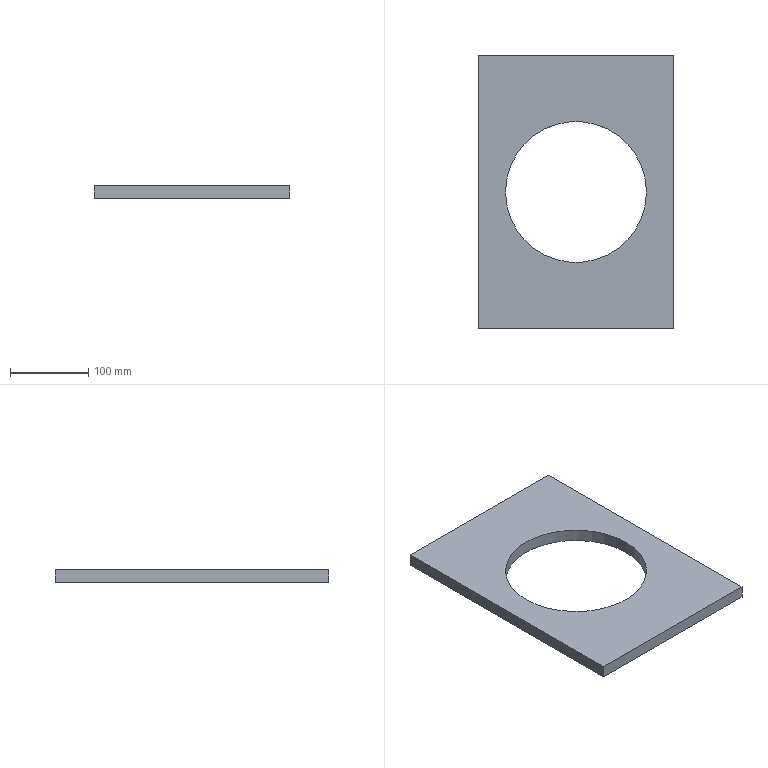Part | SolidWorks | features Extrusion 1 | 1 solid | 8 faces | box 250 x 350 x 16 mm | volume 992850 mm3 | plane 6 | cylinder 2 | commonest cylinder face diameters 180 x2
STEP:
#1=CARTESIAN_POINT('',(-90.,0.,16.));
#2=VERTEX_POINT('',#1);
#3=CARTESIAN_POINT('',(90.,0.,16.));
#4=VERTEX_POINT('',#3);
#5=CARTESIAN_POINT('',(0.,0.,16.));
#6=DIRECTION('',(0.,0.,1.));
#7=DIRECTION('',(1.,0.,0.));
#8=AXIS2_PLACEMENT_3D('',#5,#6,#7);
#9=CIRCLE('',#8,90.);
#10=EDGE_CURVE('',#2,#4,#9,.T.);
#11=ORIENTED_EDGE('',*,*,#10,.T.);
#12=CARTESIAN_POINT('',(90.,0.,0.));
#13=VERTEX_POINT('',#12);
#14=CARTESIAN_POINT('',(90.,0.,16.));
#15=DIRECTION('',(0.,0.,-1.));
#16=VECTOR('',#15,1000.);
#17=LINE('',#14,#16);
#18=EDGE_CURVE('',#4,#13,#17,.T.);
#19=ORIENTED_EDGE('',*,*,#18,.T.);
#20=CARTESIAN_POINT('',(-90.,0.,0.));
#21=VERTEX_POINT('',#20);
#22=CARTESIAN_POINT('',(0.,0.,0.));
#23=DIRECTION('',(0.,0.,1.));
#24=DIRECTION('',(1.,0.,0.));
#25=AXIS2_PLACEMENT_3D('',#22,#23,#24);
#26=CIRCLE('',#25,90.);
#27=EDGE_CURVE('',#21,#13,#26,.T.);
#28=ORIENTED_EDGE('',*,*,#27,.F.);
#29=CARTESIAN_POINT('',(-90.,0.,16.));
#30=DIRECTION('',(0.,0.,-1.));
#31=VECTOR('',#30,1000.);
#32=LINE('',#29,#31);
#33=EDGE_CURVE('',#2,#21,#32,.T.);
#34=ORIENTED_EDGE('',*,*,#33,.F.);
#35=EDGE_LOOP('',(#11,#19,#28,#34));
#36=FACE_OUTER_BOUND('',#35,.T.);
#37=CARTESIAN_POINT('',(0.,0.,16.));
#38=DIRECTION('',(0.,0.,-1.));
#39=DIRECTION('',(-1.,0.,0.));
#40=AXIS2_PLACEMENT_3D('',#37,#38,#39);
#41=CYLINDRICAL_SURFACE('',#40,90.);
#42=ADVANCED_FACE('',(#36),#41,.F.);
#43=CARTESIAN_POINT('',(-125.,175.,16.));
#44=VERTEX_POINT('',#43);
#45=CARTESIAN_POINT('',(-125.,-175.,16.));
#46=VERTEX_POINT('',#45);
#47=CARTESIAN_POINT('',(-125.,-175.,16.));
#48=DIRECTION('',(0.,-1.,0.));
#49=VECTOR('',#48,1000.);
#50=LINE('',#47,#49);
#51=EDGE_CURVE('',#44,#46,#50,.T.);
#52=ORIENTED_EDGE('',*,*,#51,.T.);
#53=CARTESIAN_POINT('',(125.,-175.,16.));
#54=VERTEX_POINT('',#53);
#55=CARTESIAN_POINT('',(125.,-175.,16.));
#56=DIRECTION('',(1.,0.,0.));
#57=VECTOR('',#56,1000.);
#58=LINE('',#55,#57);
#59=EDGE_CURVE('',#46,#54,#58,.T.);
#60=ORIENTED_EDGE('',*,*,#59,.T.);
#61=CARTESIAN_POINT('',(125.,175.,16.));
#62=VERTEX_POINT('',#61);
#63=CARTESIAN_POINT('',(125.,-175.,16.));
#64=DIRECTION('',(0.,1.,0.));
#65=VECTOR('',#64,1000.);
#66=LINE('',#63,#65);
#67=EDGE_CURVE('',#54,#62,#66,.T.);
#68=ORIENTED_EDGE('',*,*,#67,.T.);
#69=CARTESIAN_POINT('',(125.,175.,16.));
#70=DIRECTION('',(-1.,0.,0.));
#71=VECTOR('',#70,1000.);
#72=LINE('',#69,#71);
#73=EDGE_CURVE('',#62,#44,#72,.T.);
#74=ORIENTED_EDGE('',*,*,#73,.T.);
#75=EDGE_LOOP('',(#52,#60,#68,#74));
#76=FACE_OUTER_BOUND('',#75,.T.);
#77=ORIENTED_EDGE('',*,*,#10,.F.);
#78=CARTESIAN_POINT('',(0.,0.,16.));
#79=DIRECTION('',(0.,0.,1.));
#80=DIRECTION('',(1.,0.,0.));
#81=AXIS2_PLACEMENT_3D('',#78,#79,#80);
#82=CIRCLE('',#81,90.);
#83=EDGE_CURVE('',#4,#2,#82,.T.);
#84=ORIENTED_EDGE('',*,*,#83,.F.);
#85=EDGE_LOOP('',(#77,#84));
#86=FACE_BOUND('',#85,.T.);
#87=CARTESIAN_POINT('',(0.,0.,16.));
#88=DIRECTION('',(0.,0.,1.));
#89=DIRECTION('',(1.,0.,0.));
#90=AXIS2_PLACEMENT_3D('',#87,#88,#89);
#91=PLANE('',#90);
#92=ADVANCED_FACE('',(#76,#86),#91,.T.);
#93=CARTESIAN_POINT('',(-125.,175.,0.));
#94=VERTEX_POINT('',#93);
#95=CARTESIAN_POINT('',(-125.,-175.,0.));
#96=VERTEX_POINT('',#95);
#97=CARTESIAN_POINT('',(-125.,-175.,0.));
#98=DIRECTION('',(0.,-1.,0.));
#99=VECTOR('',#98,1000.);
#100=LINE('',#97,#99);
#101=EDGE_CURVE('',#94,#96,#100,.T.);
#102=ORIENTED_EDGE('',*,*,#101,.F.);
#103=CARTESIAN_POINT('',(125.,175.,0.));
#104=VERTEX_POINT('',#103);
#105=CARTESIAN_POINT('',(125.,175.,0.));
#106=DIRECTION('',(-1.,0.,0.));
#107=VECTOR('',#106,1000.);
#108=LINE('',#105,#107);
#109=EDGE_CURVE('',#104,#94,#108,.T.);
#110=ORIENTED_EDGE('',*,*,#109,.F.);
#111=CARTESIAN_POINT('',(125.,-175.,0.));
#112=VERTEX_POINT('',#111);
#113=CARTESIAN_POINT('',(125.,-175.,0.));
#114=DIRECTION('',(0.,1.,0.));
#115=VECTOR('',#114,1000.);
#116=LINE('',#113,#115);
#117=EDGE_CURVE('',#112,#104,#116,.T.);
#118=ORIENTED_EDGE('',*,*,#117,.F.);
#119=CARTESIAN_POINT('',(125.,-175.,0.));
#120=DIRECTION('',(1.,0.,0.));
#121=VECTOR('',#120,1000.);
#122=LINE('',#119,#121);
#123=EDGE_CURVE('',#96,#112,#122,.T.);
#124=ORIENTED_EDGE('',*,*,#123,.F.);
#125=EDGE_LOOP('',(#102,#110,#118,#124));
#126=FACE_OUTER_BOUND('',#125,.T.);
#127=ORIENTED_EDGE('',*,*,#27,.T.);
#128=CARTESIAN_POINT('',(0.,0.,0.));
#129=DIRECTION('',(0.,0.,1.));
#130=DIRECTION('',(1.,0.,0.));
#131=AXIS2_PLACEMENT_3D('',#128,#129,#130);
#132=CIRCLE('',#131,90.);
#133=EDGE_CURVE('',#13,#21,#132,.T.);
#134=ORIENTED_EDGE('',*,*,#133,.T.);
#135=EDGE_LOOP('',(#127,#134));
#136=FACE_BOUND('',#135,.T.);
#137=CARTESIAN_POINT('',(0.,0.,0.));
#138=DIRECTION('',(0.,0.,1.));
#139=DIRECTION('',(1.,0.,0.));
#140=AXIS2_PLACEMENT_3D('',#137,#138,#139);
#141=PLANE('',#140);
#142=ADVANCED_FACE('',(#126,#136),#141,.F.);
#143=ORIENTED_EDGE('',*,*,#101,.T.);
#144=CARTESIAN_POINT('',(-125.,-175.,16.));
#145=DIRECTION('',(0.,0.,-1.));
#146=VECTOR('',#145,1000.);
#147=LINE('',#144,#146);
#148=EDGE_CURVE('',#46,#96,#147,.T.);
#149=ORIENTED_EDGE('',*,*,#148,.F.);
#150=ORIENTED_EDGE('',*,*,#51,.F.);
#151=CARTESIAN_POINT('',(-125.,175.,16.));
#152=DIRECTION('',(0.,0.,-1.));
#153=VECTOR('',#152,1000.);
#154=LINE('',#151,#153);
#155=EDGE_CURVE('',#44,#94,#154,.T.);
#156=ORIENTED_EDGE('',*,*,#155,.T.);
#157=EDGE_LOOP('',(#143,#149,#150,#156));
#158=FACE_OUTER_BOUND('',#157,.T.);
#159=CARTESIAN_POINT('',(-125.,-175.,16.));
#160=DIRECTION('',(1.,0.,0.));
#161=DIRECTION('',(0.,0.,-1.));
#162=AXIS2_PLACEMENT_3D('',#159,#160,#161);
#163=PLANE('',#162);
#164=ADVANCED_FACE('',(#158),#163,.F.);
#165=ORIENTED_EDGE('',*,*,#123,.T.);
#166=CARTESIAN_POINT('',(125.,-175.,16.));
#167=DIRECTION('',(0.,0.,-1.));
#168=VECTOR('',#167,1000.);
#169=LINE('',#166,#168);
#170=EDGE_CURVE('',#54,#112,#169,.T.);
#171=ORIENTED_EDGE('',*,*,#170,.F.);
#172=ORIENTED_EDGE('',*,*,#59,.F.);
#173=ORIENTED_EDGE('',*,*,#148,.T.);
#174=EDGE_LOOP('',(#165,#171,#172,#173));
#175=FACE_OUTER_BOUND('',#174,.T.);
#176=CARTESIAN_POINT('',(125.,-175.,16.));
#177=DIRECTION('',(0.,1.,0.));
#178=DIRECTION('',(-1.,0.,0.));
#179=AXIS2_PLACEMENT_3D('',#176,#177,#178);
#180=PLANE('',#179);
#181=ADVANCED_FACE('',(#175),#180,.F.);
#182=ORIENTED_EDGE('',*,*,#117,.T.);
#183=CARTESIAN_POINT('',(125.,175.,16.));
#184=DIRECTION('',(0.,0.,-1.));
#185=VECTOR('',#184,1000.);
#186=LINE('',#183,#185);
#187=EDGE_CURVE('',#62,#104,#186,.T.);
#188=ORIENTED_EDGE('',*,*,#187,.F.);
#189=ORIENTED_EDGE('',*,*,#67,.F.);
#190=ORIENTED_EDGE('',*,*,#170,.T.);
#191=EDGE_LOOP('',(#182,#188,#189,#190));
#192=FACE_OUTER_BOUND('',#191,.T.);
#193=CARTESIAN_POINT('',(125.,-175.,16.));
#194=DIRECTION('',(-1.,0.,0.));
#195=DIRECTION('',(0.,0.,1.));
#196=AXIS2_PLACEMENT_3D('',#193,#194,#195);
#197=PLANE('',#196);
#198=ADVANCED_FACE('',(#192),#197,.F.);
#199=ORIENTED_EDGE('',*,*,#109,.T.);
#200=ORIENTED_EDGE('',*,*,#155,.F.);
#201=ORIENTED_EDGE('',*,*,#73,.F.);
#202=ORIENTED_EDGE('',*,*,#187,.T.);
#203=EDGE_LOOP('',(#199,#200,#201,#202));
#204=FACE_OUTER_BOUND('',#203,.T.);
#205=CARTESIAN_POINT('',(125.,175.,16.));
#206=DIRECTION('',(0.,-1.,0.));
#207=DIRECTION('',(0.,0.,-1.));
#208=AXIS2_PLACEMENT_3D('',#205,#206,#207);
#209=PLANE('',#208);
#210=ADVANCED_FACE('',(#204),#209,.F.);
#211=ORIENTED_EDGE('',*,*,#18,.F.);
#212=ORIENTED_EDGE('',*,*,#83,.T.);
#213=ORIENTED_EDGE('',*,*,#33,.T.);
#214=ORIENTED_EDGE('',*,*,#133,.F.);
#215=EDGE_LOOP('',(#211,#212,#213,#214));
#216=FACE_OUTER_BOUND('',#215,.T.);
#217=CARTESIAN_POINT('',(0.,0.,16.));
#218=DIRECTION('',(0.,0.,-1.));
#219=DIRECTION('',(-1.,0.,0.));
#220=AXIS2_PLACEMENT_3D('',#217,#218,#219);
#221=CYLINDRICAL_SURFACE('',#220,90.);
#222=ADVANCED_FACE('',(#216),#221,.F.);
#223=CLOSED_SHELL('',(#42,#92,#142,#164,#181,#198,#210,#222));
#224=MANIFOLD_SOLID_BREP('',#223);
#225=CARTESIAN_POINT('',(0.,0.,0.));
#226=DIRECTION('',(0.,0.,1.));
#227=DIRECTION('',(1.,0.,0.));
#228=AXIS2_PLACEMENT_3D('',#225,#226,#227);
#229=(LENGTH_UNIT()NAMED_UNIT(*)SI_UNIT(.MILLI.,.METRE.));
#230=UNCERTAINTY_MEASURE_WITH_UNIT(LENGTH_MEASURE(0.00001),#229,'','');
#231=(NAMED_UNIT(*)PLANE_ANGLE_UNIT()SI_UNIT($,.RADIAN.));
#232=(NAMED_UNIT(*)SI_UNIT($,.STERADIAN.)SOLID_ANGLE_UNIT());
#233=(GEOMETRIC_REPRESENTATION_CONTEXT(3)GLOBAL_UNCERTAINTY_ASSIGNED_CONTEXT((#230))GLOBAL_UNIT_ASSIGNED_CONTEXT((#229,#231,#232))REPRESENTATION_CONTEXT('',''));
#234=ADVANCED_BREP_SHAPE_REPRESENTATION('',(#224,#228),#233);